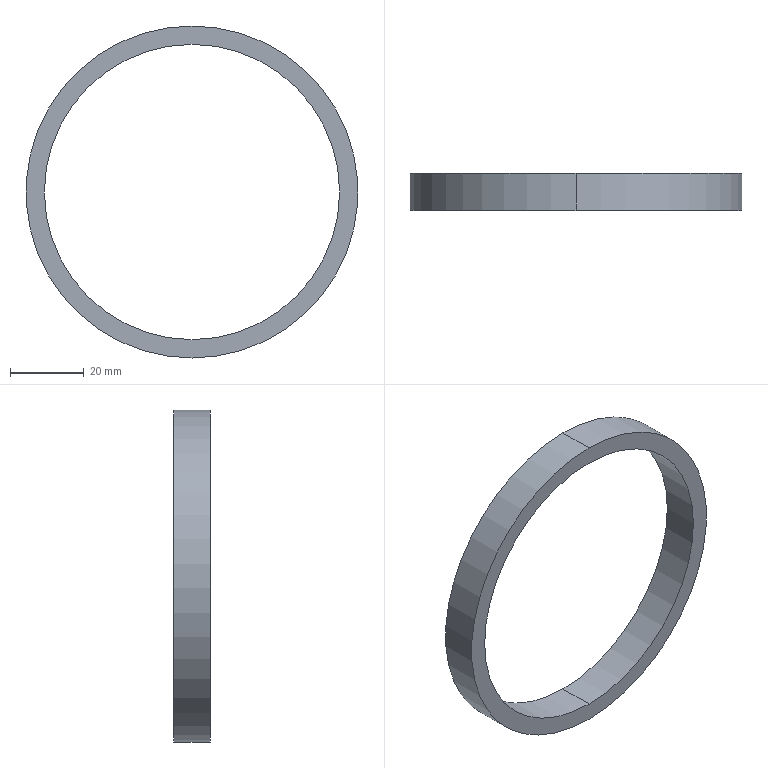Part | SolidWorks | features BaseBody 1 | 1 solid | 6 faces | box 90 x 10 x 90 mm | volume 13352 mm3 | cylinder 4 | plane 2 | commonest cylinder face diameters 80 x2 90 x2
STEP:
#1=CARTESIAN_POINT('',(0.,10.,-45.));
#2=VERTEX_POINT('',#1);
#3=CARTESIAN_POINT('',(0.,10.,45.));
#4=VERTEX_POINT('',#3);
#5=CARTESIAN_POINT('',(0.,10.,0.));
#6=DIRECTION('',(0.,-1.,0.));
#7=DIRECTION('',(0.,0.,-1.));
#8=AXIS2_PLACEMENT_3D('',#5,#6,#7);
#9=CIRCLE('',#8,45.);
#10=EDGE_CURVE('',#2,#4,#9,.T.);
#11=ORIENTED_EDGE('',*,*,#10,.T.);
#12=CARTESIAN_POINT('',(0.,0.,45.));
#13=VERTEX_POINT('',#12);
#14=CARTESIAN_POINT('',(0.,10.,45.));
#15=DIRECTION('',(0.,-1.,0.));
#16=VECTOR('',#15,1000.);
#17=LINE('',#14,#16);
#18=EDGE_CURVE('',#4,#13,#17,.T.);
#19=ORIENTED_EDGE('',*,*,#18,.T.);
#20=CARTESIAN_POINT('',(0.,0.,-45.));
#21=VERTEX_POINT('',#20);
#22=CARTESIAN_POINT('',(0.,0.,0.));
#23=DIRECTION('',(0.,1.,0.));
#24=DIRECTION('',(0.,0.,-1.));
#25=AXIS2_PLACEMENT_3D('',#22,#23,#24);
#26=CIRCLE('',#25,45.);
#27=EDGE_CURVE('',#13,#21,#26,.T.);
#28=ORIENTED_EDGE('',*,*,#27,.T.);
#29=CARTESIAN_POINT('',(0.,10.,-45.));
#30=DIRECTION('',(0.,-1.,0.));
#31=VECTOR('',#30,1000.);
#32=LINE('',#29,#31);
#33=EDGE_CURVE('',#2,#21,#32,.T.);
#34=ORIENTED_EDGE('',*,*,#33,.F.);
#35=EDGE_LOOP('',(#11,#19,#28,#34));
#36=FACE_OUTER_BOUND('',#35,.T.);
#37=CARTESIAN_POINT('',(0.,10.,0.));
#38=DIRECTION('',(0.,-1.,0.));
#39=DIRECTION('',(0.,0.,-1.));
#40=AXIS2_PLACEMENT_3D('',#37,#38,#39);
#41=CYLINDRICAL_SURFACE('',#40,45.);
#42=ADVANCED_FACE('',(#36),#41,.T.);
#43=CARTESIAN_POINT('',(0.,10.,40.));
#44=VERTEX_POINT('',#43);
#45=CARTESIAN_POINT('',(0.,10.,-40.));
#46=VERTEX_POINT('',#45);
#47=CARTESIAN_POINT('',(0.,10.,0.));
#48=DIRECTION('',(0.,-1.,0.));
#49=DIRECTION('',(0.,0.,-1.));
#50=AXIS2_PLACEMENT_3D('',#47,#48,#49);
#51=CIRCLE('',#50,40.);
#52=EDGE_CURVE('',#44,#46,#51,.T.);
#53=ORIENTED_EDGE('',*,*,#52,.F.);
#54=CARTESIAN_POINT('',(0.,0.,40.));
#55=VERTEX_POINT('',#54);
#56=CARTESIAN_POINT('',(0.,10.,40.));
#57=DIRECTION('',(0.,-1.,0.));
#58=VECTOR('',#57,1000.);
#59=LINE('',#56,#58);
#60=EDGE_CURVE('',#44,#55,#59,.T.);
#61=ORIENTED_EDGE('',*,*,#60,.T.);
#62=CARTESIAN_POINT('',(0.,0.,-40.));
#63=VERTEX_POINT('',#62);
#64=CARTESIAN_POINT('',(0.,0.,0.));
#65=DIRECTION('',(0.,-1.,0.));
#66=DIRECTION('',(0.,0.,-1.));
#67=AXIS2_PLACEMENT_3D('',#64,#65,#66);
#68=CIRCLE('',#67,40.);
#69=EDGE_CURVE('',#55,#63,#68,.T.);
#70=ORIENTED_EDGE('',*,*,#69,.T.);
#71=CARTESIAN_POINT('',(0.,10.,-40.));
#72=DIRECTION('',(0.,-1.,0.));
#73=VECTOR('',#72,1000.);
#74=LINE('',#71,#73);
#75=EDGE_CURVE('',#46,#63,#74,.T.);
#76=ORIENTED_EDGE('',*,*,#75,.F.);
#77=EDGE_LOOP('',(#53,#61,#70,#76));
#78=FACE_OUTER_BOUND('',#77,.T.);
#79=CARTESIAN_POINT('',(0.,10.,0.));
#80=DIRECTION('',(0.,-1.,0.));
#81=DIRECTION('',(0.,0.,-1.));
#82=AXIS2_PLACEMENT_3D('',#79,#80,#81);
#83=CYLINDRICAL_SURFACE('',#82,40.);
#84=ADVANCED_FACE('',(#78),#83,.F.);
#85=ORIENTED_EDGE('',*,*,#18,.F.);
#86=CARTESIAN_POINT('',(0.,10.,0.));
#87=DIRECTION('',(0.,-1.,0.));
#88=DIRECTION('',(0.,0.,-1.));
#89=AXIS2_PLACEMENT_3D('',#86,#87,#88);
#90=CIRCLE('',#89,45.);
#91=EDGE_CURVE('',#4,#2,#90,.T.);
#92=ORIENTED_EDGE('',*,*,#91,.T.);
#93=ORIENTED_EDGE('',*,*,#33,.T.);
#94=CARTESIAN_POINT('',(0.,0.,0.));
#95=DIRECTION('',(0.,1.,0.));
#96=DIRECTION('',(0.,0.,-1.));
#97=AXIS2_PLACEMENT_3D('',#94,#95,#96);
#98=CIRCLE('',#97,45.);
#99=EDGE_CURVE('',#21,#13,#98,.T.);
#100=ORIENTED_EDGE('',*,*,#99,.T.);
#101=EDGE_LOOP('',(#85,#92,#93,#100));
#102=FACE_OUTER_BOUND('',#101,.T.);
#103=CARTESIAN_POINT('',(0.,10.,0.));
#104=DIRECTION('',(0.,-1.,0.));
#105=DIRECTION('',(0.,0.,-1.));
#106=AXIS2_PLACEMENT_3D('',#103,#104,#105);
#107=CYLINDRICAL_SURFACE('',#106,45.);
#108=ADVANCED_FACE('',(#102),#107,.T.);
#109=CARTESIAN_POINT('',(0.,0.,0.));
#110=DIRECTION('',(0.,-1.,0.));
#111=DIRECTION('',(0.,0.,-1.));
#112=AXIS2_PLACEMENT_3D('',#109,#110,#111);
#113=CIRCLE('',#112,40.);
#114=EDGE_CURVE('',#63,#55,#113,.T.);
#115=ORIENTED_EDGE('',*,*,#114,.F.);
#116=ORIENTED_EDGE('',*,*,#69,.F.);
#117=EDGE_LOOP('',(#115,#116));
#118=FACE_BOUND('',#117,.T.);
#119=ORIENTED_EDGE('',*,*,#99,.F.);
#120=ORIENTED_EDGE('',*,*,#27,.F.);
#121=EDGE_LOOP('',(#119,#120));
#122=FACE_OUTER_BOUND('',#121,.T.);
#123=CARTESIAN_POINT('',(0.,0.,0.));
#124=DIRECTION('',(0.,1.,0.));
#125=DIRECTION('',(0.,0.,1.));
#126=AXIS2_PLACEMENT_3D('',#123,#124,#125);
#127=PLANE('',#126);
#128=ADVANCED_FACE('',(#118,#122),#127,.F.);
#129=CARTESIAN_POINT('',(0.,10.,0.));
#130=DIRECTION('',(0.,-1.,0.));
#131=DIRECTION('',(0.,0.,-1.));
#132=AXIS2_PLACEMENT_3D('',#129,#130,#131);
#133=CIRCLE('',#132,40.);
#134=EDGE_CURVE('',#46,#44,#133,.T.);
#135=ORIENTED_EDGE('',*,*,#134,.T.);
#136=ORIENTED_EDGE('',*,*,#52,.T.);
#137=EDGE_LOOP('',(#135,#136));
#138=FACE_BOUND('',#137,.T.);
#139=ORIENTED_EDGE('',*,*,#10,.F.);
#140=ORIENTED_EDGE('',*,*,#91,.F.);
#141=EDGE_LOOP('',(#139,#140));
#142=FACE_OUTER_BOUND('',#141,.T.);
#143=CARTESIAN_POINT('',(0.,10.,0.));
#144=DIRECTION('',(0.,1.,0.));
#145=DIRECTION('',(0.,0.,1.));
#146=AXIS2_PLACEMENT_3D('',#143,#144,#145);
#147=PLANE('',#146);
#148=ADVANCED_FACE('',(#138,#142),#147,.T.);
#149=ORIENTED_EDGE('',*,*,#60,.F.);
#150=ORIENTED_EDGE('',*,*,#134,.F.);
#151=ORIENTED_EDGE('',*,*,#75,.T.);
#152=ORIENTED_EDGE('',*,*,#114,.T.);
#153=EDGE_LOOP('',(#149,#150,#151,#152));
#154=FACE_OUTER_BOUND('',#153,.T.);
#155=CARTESIAN_POINT('',(0.,10.,0.));
#156=DIRECTION('',(0.,-1.,0.));
#157=DIRECTION('',(0.,0.,-1.));
#158=AXIS2_PLACEMENT_3D('',#155,#156,#157);
#159=CYLINDRICAL_SURFACE('',#158,40.);
#160=ADVANCED_FACE('',(#154),#159,.F.);
#161=CLOSED_SHELL('',(#42,#84,#108,#128,#148,#160));
#162=MANIFOLD_SOLID_BREP('',#161);
#163=CARTESIAN_POINT('',(0.,0.,0.));
#164=DIRECTION('',(0.,0.,1.));
#165=DIRECTION('',(1.,0.,0.));
#166=AXIS2_PLACEMENT_3D('',#163,#164,#165);
#167=(LENGTH_UNIT()NAMED_UNIT(*)SI_UNIT(.MILLI.,.METRE.));
#168=UNCERTAINTY_MEASURE_WITH_UNIT(LENGTH_MEASURE(0.00001),#167,'','');
#169=(NAMED_UNIT(*)PLANE_ANGLE_UNIT()SI_UNIT($,.RADIAN.));
#170=(NAMED_UNIT(*)SI_UNIT($,.STERADIAN.)SOLID_ANGLE_UNIT());
#171=(GEOMETRIC_REPRESENTATION_CONTEXT(3)GLOBAL_UNCERTAINTY_ASSIGNED_CONTEXT((#168))GLOBAL_UNIT_ASSIGNED_CONTEXT((#167,#169,#170))REPRESENTATION_CONTEXT('',''));
#172=ADVANCED_BREP_SHAPE_REPRESENTATION('',(#162,#166),#171);